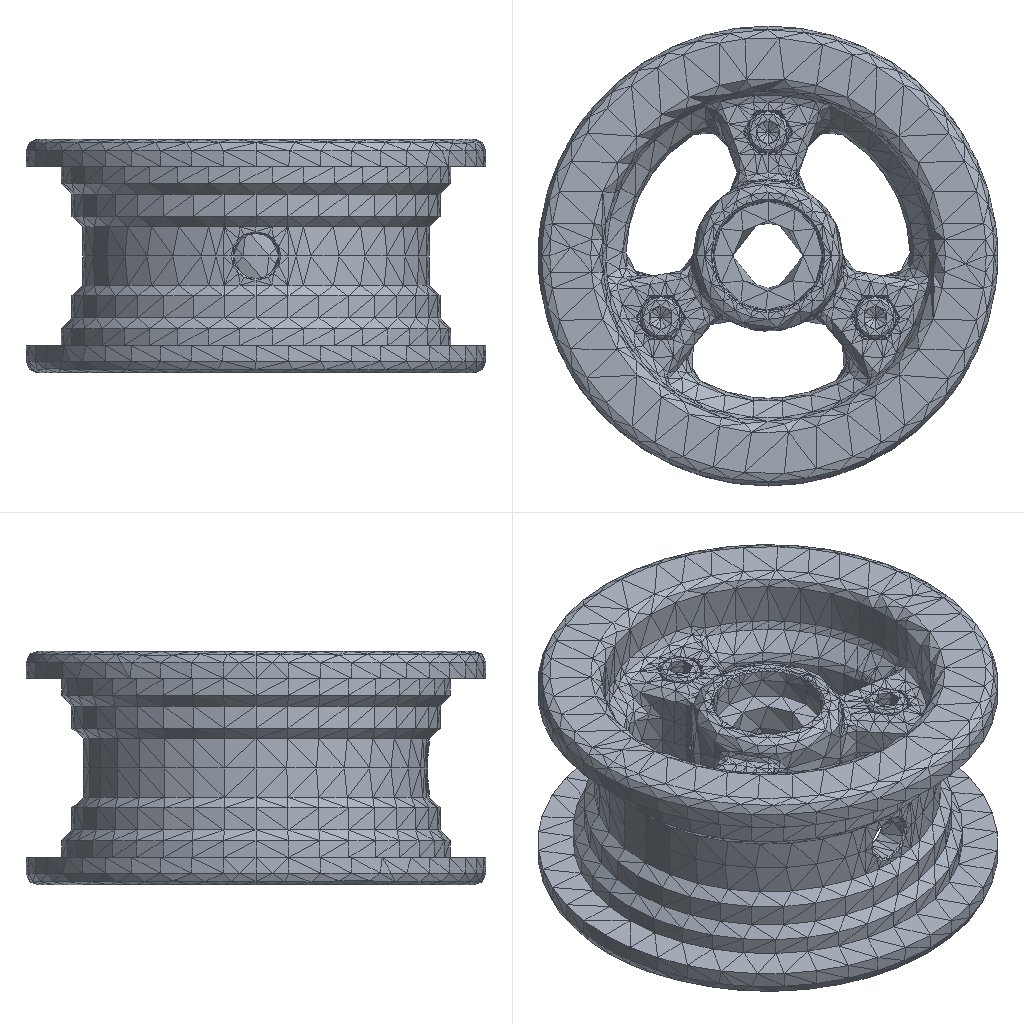Simulation study | ansys workbench
Set-up summary:
category,name,step,type,value,unit,region
solver,ansys_workbench
units,mm-N-s-tonne (MPa),,stated,"/units,MPA"
analysis,deck-1/LS1,,modal,method=lanb; n_modes=6
load_step,deck-1/LS1,deck-1/LS1,modal
analysis,deck-2/LS1,,static
load_step,deck-2/LS1,deck-2/LS1,static,nsubst=1; time=1
analysis,deck-3/LS1,,static
load_step,deck-3/LS1,deck-3/LS1,static,nsubst=1; time=1
analysis,deck-4/LS1,,static
load_step,deck-4/LS1,deck-4/LS1,static,nsubst=1; time=1
analysis,deck-5/LS1,,static
load_step,deck-5/LS1,deck-5/LS1,static,nsubst=1; time=1
mesh,deck-1.dat,,nodes,34656
mesh,deck-1.dat,,elements,21920
element_type,SOLID187,,,18532,,deck-1.dat
element_type,TARGE170,,,1694,,deck-1.dat
element_type,CONTA174,,,1694,,deck-1.dat
mesh,deck-2.dat,,nodes,34657
mesh,deck-2.dat,,elements,22242
element_type,SOLID187,,,18532,,deck-2.dat
element_type,CONTA174,,,2016,,deck-2.dat
element_type,TARGE170,,,1694,,deck-2.dat
mesh,deck-3.dat,,nodes,34657
mesh,deck-3.dat,,elements,22221
element_type,SOLID187,,,18532,,deck-3.dat
element_type,CONTA174,,,1995,,deck-3.dat
element_type,TARGE170,,,1694,,deck-3.dat
mesh,deck-4.dat,,nodes,24093
mesh,deck-4.dat,,elements,14349
element_type,SOLID187,,,12870,,deck-4.dat
element_type,CONTA174,,,879,,deck-4.dat
element_type,TARGE170,,,600,,deck-4.dat
mesh,deck-5.dat,,nodes,24093
mesh,deck-5.dat,,elements,14272
element_type,SOLID187,,,12870,,deck-5.dat
element_type,CONTA174,,,802,,deck-5.dat
element_type,TARGE170,,,600,,deck-5.dat
material,Structural Steel,,E,200000,tonne s^-2 mm^-1
material,Structural Steel,,nu,0.3
material,Structural Steel,,density,7.85e-09,tonne mm^-3
material,Structural Steel,,conductivity,60.5,tonne mm s^-3 C^-1
material,Structural Steel,,specific_heat,4.34e+08,mm^2 s^-2 C^-1
material,Structural Steel,,cte,1.2e-05,C^-1
material,Structural Steel,,permeability,10000
material,Structural Steel,,resistivity,0.00017,ohm mm
material,Structural Steel,,E,200000,tonne s^-2 mm^-1
material,Structural Steel,,nu,0.3
material,Structural Steel,,density,7.85e-09,tonne mm^-3
material,Structural Steel,,conductivity,60.5,tonne mm s^-3 C^-1
material,Structural Steel,,specific_heat,4.34e+08,mm^2 s^-2 C^-1
material,Structural Steel,,cte,1.2e-05,C^-1
material,Structural Steel,,permeability,10000
material,Structural Steel,,resistivity,0.00017,ohm mm
material,6061,,E,200000,tonne s^-2 mm^-1
material,6061,,nu,0.3
material,6061,,density,7.85e-09,tonne mm^-3
material,6061,,conductivity,60.5,tonne mm s^-3 C^-1
material,6061,,specific_heat,4.34e+08,mm^2 s^-2 C^-1
material,6061,,cte,1.2e-05,C^-1
material,6061,,permeability,10000
material,6061,,resistivity,0.00017,ohm mm
material,Structural Steel,,E,200000,tonne s^-2 mm^-1
material,Structural Steel,,nu,0.3
material,Structural Steel,,density,7.85e-09,tonne mm^-3
material,Structural Steel,,conductivity,60.5,tonne mm s^-3 C^-1
material,Structural Steel,,specific_heat,4.34e+08,mm^2 s^-2 C^-1
material,Structural Steel,,cte,1.2e-05,C^-1
material,Structural Steel,,permeability,10000
material,Structural Steel,,resistivity,0.00017,ohm mm
material,6061,,E,200000,tonne s^-2 mm^-1
material,6061,,nu,0.3
material,6061,,density,7.85e-09,tonne mm^-3
material,6061,,conductivity,60.5,tonne mm s^-3 C^-1
material,6061,,specific_heat,4.34e+08,mm^2 s^-2 C^-1
material,6061,,cte,1.2e-05,C^-1
material,6061,,permeability,10000
material,6061,,resistivity,0.00017,ohm mm
load,,deck-2/LS1,moment,"5000 [dir=(0, 0, 1) n=3]",,all
load,,deck-3/LS1,moment,"50000 [dir=(0, 0, 1) n=3]",,all
load,,deck-4/LS1,moment,"5000 [dir=(0, 0, 1) n=3]",,all
load,,deck-5/LS1,moment,"50000 [dir=(0, 0, 1) n=3]",,all
bc,Fixed Supports,deck-2/model,fixed,[dofs=ALL],,_FIXEDSU
bc,Fixed Supports,deck-3/model,fixed,[dofs=ALL],,_FIXEDSU
bc,Fixed Supports,deck-4/model,fixed,[dofs=ALL],,_FIXEDSU
bc,Fixed Supports,deck-5/model,fixed,[dofs=ALL],,_FIXEDSU
contact,Contact Region,,bonded (always),element=CONTA174
contact,Contact Region 2,,bonded (always),element=CONTA174
contact,Contact Region 3,,bonded (always),element=CONTA174
contact,Contact Region 4,,bonded (always),element=CONTA174
contact,Contact Region 5,,bonded (always),element=CONTA174
contact,Contact Region 6,,bonded (always),element=CONTA174
contact,Contact Region 7,,bonded (always),element=CONTA174
contact,Contact Region,,bonded (always),element=CONTA174
contact,Contact Region 2,,bonded (always),element=CONTA174
contact,Contact Region 3,,bonded (always),element=CONTA174
contact,Contact Region 4,,bonded (always),element=CONTA174
contact,Contact Region 5,,bonded (always),element=CONTA174
contact,Contact Region 6,,bonded (always),element=CONTA174
contact,Contact Region 7,,bonded (always),element=CONTA174
contact,contact 8,,bonded (always),element=CONTA174
contact,Contact Region,,bonded (always),element=CONTA174
contact,Contact Region 2,,bonded (always),element=CONTA174
contact,Contact Region 3,,bonded (always),element=CONTA174
contact,Contact Region 4,,bonded (always),element=CONTA174
contact,Contact Region 5,,bonded (always),element=CONTA174
contact,Contact Region 6,,bonded (always),element=CONTA174
contact,Contact Region 7,,bonded (always),element=CONTA174
contact,contact 8,,bonded (always),element=CONTA174
contact,Contact Region,,bonded (always),element=CONTA174
contact,contact 2,,bonded (always),element=CONTA174
contact,Contact Region,,bonded (always),element=CONTA174
contact,contact 2,,bonded (always),element=CONTA174
named_set,_FIXEDSU,,node,538
named_set,_FIXEDSU,,node,507
named_set,_FIXEDSU,,node,128
named_set,_FIXEDSU,,node,128
Results summary:
result,analyses[0].index,,,1
result,analyses[0].system,,,SYS
result,analyses[0].deck,,,deck-1.dat
result,analyses[0].solve_status,,,completed
result,analyses[0].analysis_type,,,modal
result,analyses[0].physics,,,mechanical
result,analyses[0].unit_system,,,"NMM: mm, ton, N, s, mV, mA, degC"
result,analyses[0].n_sets,,,6
result,analyses[0].modal_frequencies_hz[1],,,0
result,analyses[0].modal_frequencies_hz[2],,,0.004962
result,analyses[0].modal_frequencies_hz[3],,,0.007047
result,analyses[0].modal_frequencies_hz[4],,,149.096
result,analyses[0].modal_frequencies_hz[5],,,167.127
result,analyses[0].modal_frequencies_hz[6],,,171.661
result,analyses[1].index,,,2
result,analyses[1].system,,,SYS-1
result,analyses[1].deck,,,deck-2.dat
result,analyses[1].solve_status,,,completed
result,analyses[1].analysis_type,,,static
result,analyses[1].physics,,,mechanical
result,analyses[1].unit_system,,,"NMM: mm, ton, N, s, mV, mA, degC"
result,analyses[1].n_sets,,,1
result,analyses[1].load_steps[0].set,set=1,,1
result,analyses[1].load_steps[0].time_or_freq,set=1,,1
result,analyses[1].load_steps[0].max_displacement_magnitude,set=1,,0.0001512
result,analyses[1].load_steps[0].max_von_mises_nodal,set=1,,16.363
result,analyses[1].load_steps[0].reaction_force_sum_xyz[1],set=1,,9.11178e-10
result,analyses[1].load_steps[0].reaction_force_sum_xyz[2],set=1,,-5.13359e-08
result,analyses[1].load_steps[0].reaction_force_sum_xyz[3],set=1,,4.70492e-08
result,analyses[2].index,,,3
result,analyses[2].system,,,SYS-2
result,analyses[2].deck,,,deck-3.dat
result,analyses[2].solve_status,,,completed
result,analyses[2].analysis_type,,,static
result,analyses[2].physics,,,mechanical
result,analyses[2].unit_system,,,"NMM: mm, ton, N, s, mV, mA, degC"
result,analyses[2].n_sets,,,1
result,analyses[2].load_steps[0].set,set=1,,1
result,analyses[2].load_steps[0].time_or_freq,set=1,,1
result,analyses[2].load_steps[0].max_displacement_magnitude,set=1,,0.001488
result,analyses[2].load_steps[0].max_von_mises_nodal,set=1,,156.338
result,analyses[2].load_steps[0].reaction_force_sum_xyz[1],set=1,,2.6277e-06
result,analyses[2].load_steps[0].reaction_force_sum_xyz[2],set=1,,-1.33143e-06
result,analyses[2].load_steps[0].reaction_force_sum_xyz[3],set=1,,1.63679e-06
result,analyses[3].index,,,4
result,analyses[3].system,,,SYS-3
result,analyses[3].deck,,,deck-4.dat
result,analyses[3].solve_status,,,completed
result,analyses[3].analysis_type,,,static
result,analyses[3].physics,,,mechanical
result,analyses[3].unit_system,,,"NMM: mm, ton, N, s, mV, mA, degC"
result,analyses[3].n_sets,,,1
result,analyses[3].load_steps[0].set,set=1,,1
result,analyses[3].load_steps[0].time_or_freq,set=1,,1
result,analyses[3].load_steps[0].max_displacement_magnitude,set=1,,0.0004058
result,analyses[3].load_steps[0].max_von_mises_nodal,set=1,,1.18
result,analyses[3].load_steps[0].reaction_force_sum_xyz[1],set=1,,2.35621e-07
result,analyses[3].load_steps[0].reaction_force_sum_xyz[2],set=1,,2.09992e-07
result,analyses[3].load_steps[0].reaction_force_sum_xyz[3],set=1,,-2.10005e-07
result,analyses[4].index,,,5
result,analyses[4].system,,,SYS-4
result,analyses[4].deck,,,deck-5.dat
result,analyses[4].solve_status,,,completed
result,analyses[4].analysis_type,,,static
result,analyses[4].physics,,,mechanical
result,analyses[4].unit_system,,,"NMM: mm, ton, N, s, mV, mA, degC"
result,analyses[4].n_sets,,,1
result,analyses[4].load_steps[0].set,set=1,,1
result,analyses[4].load_steps[0].time_or_freq,set=1,,1
result,analyses[4].load_steps[0].max_displacement_magnitude,set=1,,0.004034
result,analyses[4].load_steps[0].max_von_mises_nodal,set=1,,11.933
result,analyses[4].load_steps[0].reaction_force_sum_xyz[1],set=1,,-2.46514e-06
result,analyses[4].load_steps[0].reaction_force_sum_xyz[2],set=1,,1.41e-06
result,analyses[4].load_steps[0].reaction_force_sum_xyz[3],set=1,,-1.64044e-06